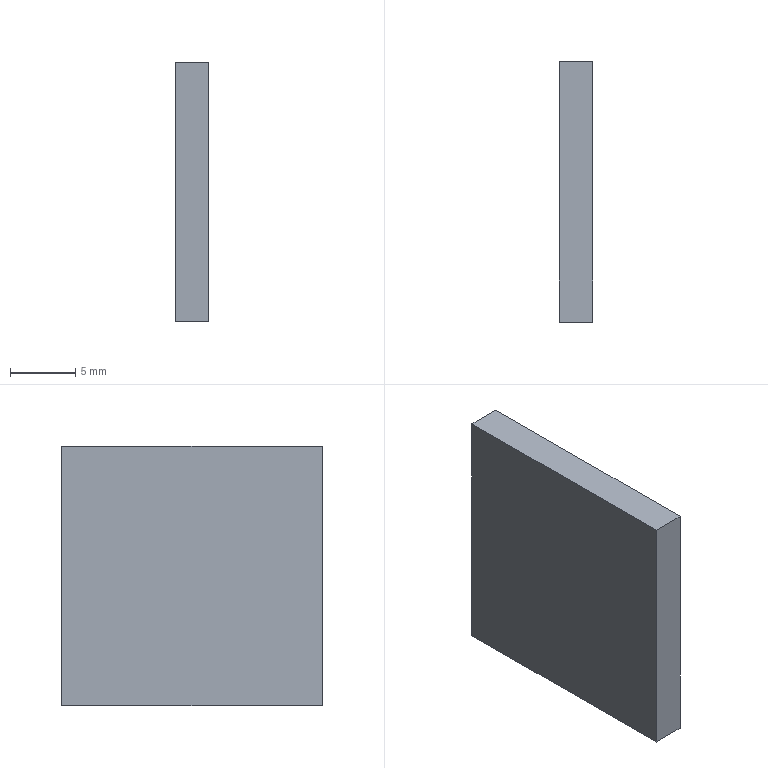Part | NX | features .2 2 | 1 solid | 6 faces | box 2.595 x 20 x 19.901 mm | volume 1033 mm3 | plane 6
STEP:
#1=CARTESIAN_POINT('',(-1240.065,-525.,-424.024));
#2=VERTEX_POINT('',#1);
#3=CARTESIAN_POINT('',(-1240.065,-545.,-424.024));
#4=VERTEX_POINT('',#3);
#5=CARTESIAN_POINT('',(-1240.065,-535.,-424.024));
#6=DIRECTION('',(0.,-1.,0.));
#7=VECTOR('',#6,1000.);
#8=LINE('',#5,#7);
#9=EDGE_CURVE('',#2,#4,#8,.T.);
#10=ORIENTED_EDGE('',*,*,#9,.F.);
#11=CARTESIAN_POINT('',(-1237.47,-525.,-424.024));
#12=VERTEX_POINT('',#11);
#13=CARTESIAN_POINT('',(-1238.768,-525.,-424.024));
#14=DIRECTION('',(1.,0.,0.));
#15=VECTOR('',#14,1000.);
#16=LINE('',#13,#15);
#17=EDGE_CURVE('',#2,#12,#16,.T.);
#18=ORIENTED_EDGE('',*,*,#17,.T.);
#19=CARTESIAN_POINT('',(-1237.47,-545.,-424.024));
#20=VERTEX_POINT('',#19);
#21=CARTESIAN_POINT('',(-1237.47,-535.,-424.024));
#22=DIRECTION('',(0.,-1.,0.));
#23=VECTOR('',#22,1000.);
#24=LINE('',#21,#23);
#25=EDGE_CURVE('',#12,#20,#24,.T.);
#26=ORIENTED_EDGE('',*,*,#25,.T.);
#27=CARTESIAN_POINT('',(-1238.768,-545.,-424.024));
#28=DIRECTION('',(1.,0.,0.));
#29=VECTOR('',#28,1000.);
#30=LINE('',#27,#29);
#31=EDGE_CURVE('',#4,#20,#30,.T.);
#32=ORIENTED_EDGE('',*,*,#31,.F.);
#33=EDGE_LOOP('',(#10,#18,#26,#32));
#34=FACE_BOUND('',#33,.T.);
#35=CARTESIAN_POINT('',(-1237.47,-535.,-424.024));
#36=DIRECTION('',(0.,0.,1.));
#37=DIRECTION('',(-1.,0.,0.));
#38=AXIS2_PLACEMENT_3D('',#35,#36,#37);
#39=PLANE('',#38);
#40=ADVANCED_FACE('',(#34),#39,.F.);
#41=ORIENTED_EDGE('',*,*,#25,.F.);
#42=CARTESIAN_POINT('',(-1237.47,-525.,-404.124));
#43=VERTEX_POINT('',#42);
#44=CARTESIAN_POINT('',(-1237.47,-525.,-414.074));
#45=DIRECTION('',(0.,0.,1.));
#46=VECTOR('',#45,1000.);
#47=LINE('',#44,#46);
#48=EDGE_CURVE('',#12,#43,#47,.T.);
#49=ORIENTED_EDGE('',*,*,#48,.T.);
#50=CARTESIAN_POINT('',(-1237.47,-545.,-404.124));
#51=VERTEX_POINT('',#50);
#52=CARTESIAN_POINT('',(-1237.47,-535.,-404.124));
#53=DIRECTION('',(0.,-1.,0.));
#54=VECTOR('',#53,1000.);
#55=LINE('',#52,#54);
#56=EDGE_CURVE('',#43,#51,#55,.T.);
#57=ORIENTED_EDGE('',*,*,#56,.T.);
#58=CARTESIAN_POINT('',(-1237.47,-545.,-414.074));
#59=DIRECTION('',(0.,0.,1.));
#60=VECTOR('',#59,1000.);
#61=LINE('',#58,#60);
#62=EDGE_CURVE('',#20,#51,#61,.T.);
#63=ORIENTED_EDGE('',*,*,#62,.F.);
#64=EDGE_LOOP('',(#41,#49,#57,#63));
#65=FACE_BOUND('',#64,.T.);
#66=CARTESIAN_POINT('',(-1237.47,-535.,-404.124));
#67=DIRECTION('',(-1.,0.,0.));
#68=DIRECTION('',(0.,0.,-1.));
#69=AXIS2_PLACEMENT_3D('',#66,#67,#68);
#70=PLANE('',#69);
#71=ADVANCED_FACE('',(#65),#70,.F.);
#72=ORIENTED_EDGE('',*,*,#56,.F.);
#73=CARTESIAN_POINT('',(-1240.065,-525.,-404.124));
#74=VERTEX_POINT('',#73);
#75=CARTESIAN_POINT('',(-1238.768,-525.,-404.124));
#76=DIRECTION('',(-1.,0.,0.));
#77=VECTOR('',#76,1000.);
#78=LINE('',#75,#77);
#79=EDGE_CURVE('',#43,#74,#78,.T.);
#80=ORIENTED_EDGE('',*,*,#79,.T.);
#81=CARTESIAN_POINT('',(-1240.065,-545.,-404.124));
#82=VERTEX_POINT('',#81);
#83=CARTESIAN_POINT('',(-1240.065,-535.,-404.124));
#84=DIRECTION('',(0.,-1.,0.));
#85=VECTOR('',#84,1000.);
#86=LINE('',#83,#85);
#87=EDGE_CURVE('',#74,#82,#86,.T.);
#88=ORIENTED_EDGE('',*,*,#87,.T.);
#89=CARTESIAN_POINT('',(-1238.768,-545.,-404.124));
#90=DIRECTION('',(-1.,0.,0.));
#91=VECTOR('',#90,1000.);
#92=LINE('',#89,#91);
#93=EDGE_CURVE('',#51,#82,#92,.T.);
#94=ORIENTED_EDGE('',*,*,#93,.F.);
#95=EDGE_LOOP('',(#72,#80,#88,#94));
#96=FACE_BOUND('',#95,.T.);
#97=CARTESIAN_POINT('',(-1245.159,-535.,-404.124));
#98=DIRECTION('',(0.,0.,-1.));
#99=DIRECTION('',(1.,0.,0.));
#100=AXIS2_PLACEMENT_3D('',#97,#98,#99);
#101=PLANE('',#100);
#102=ADVANCED_FACE('',(#96),#101,.F.);
#103=ORIENTED_EDGE('',*,*,#87,.F.);
#104=CARTESIAN_POINT('',(-1240.065,-525.,-414.074));
#105=DIRECTION('',(0.,0.,-1.));
#106=VECTOR('',#105,1000.);
#107=LINE('',#104,#106);
#108=EDGE_CURVE('',#74,#2,#107,.T.);
#109=ORIENTED_EDGE('',*,*,#108,.T.);
#110=ORIENTED_EDGE('',*,*,#9,.T.);
#111=CARTESIAN_POINT('',(-1240.065,-545.,-414.074));
#112=DIRECTION('',(0.,0.,-1.));
#113=VECTOR('',#112,1000.);
#114=LINE('',#111,#113);
#115=EDGE_CURVE('',#82,#4,#114,.T.);
#116=ORIENTED_EDGE('',*,*,#115,.F.);
#117=EDGE_LOOP('',(#103,#109,#110,#116));
#118=FACE_BOUND('',#117,.T.);
#119=CARTESIAN_POINT('',(-1240.065,-535.,-424.024));
#120=DIRECTION('',(1.,0.,0.));
#121=DIRECTION('',(0.,0.,1.));
#122=AXIS2_PLACEMENT_3D('',#119,#120,#121);
#123=PLANE('',#122);
#124=ADVANCED_FACE('',(#118),#123,.F.);
#125=ORIENTED_EDGE('',*,*,#108,.F.);
#126=ORIENTED_EDGE('',*,*,#79,.F.);
#127=ORIENTED_EDGE('',*,*,#48,.F.);
#128=ORIENTED_EDGE('',*,*,#17,.F.);
#129=EDGE_LOOP('',(#125,#126,#127,#128));
#130=FACE_BOUND('',#129,.T.);
#131=CARTESIAN_POINT('',(-1141.,-525.,-500.));
#132=DIRECTION('',(0.,-1.,0.));
#133=DIRECTION('',(-1.,0.,0.));
#134=AXIS2_PLACEMENT_3D('',#131,#132,#133);
#135=PLANE('',#134);
#136=ADVANCED_FACE('',(#130),#135,.F.);
#137=ORIENTED_EDGE('',*,*,#31,.T.);
#138=ORIENTED_EDGE('',*,*,#62,.T.);
#139=ORIENTED_EDGE('',*,*,#93,.T.);
#140=ORIENTED_EDGE('',*,*,#115,.T.);
#141=EDGE_LOOP('',(#137,#138,#139,#140));
#142=FACE_BOUND('',#141,.T.);
#143=CARTESIAN_POINT('',(-1141.,-545.,-500.));
#144=DIRECTION('',(0.,-1.,0.));
#145=DIRECTION('',(-1.,0.,0.));
#146=AXIS2_PLACEMENT_3D('',#143,#144,#145);
#147=PLANE('',#146);
#148=ADVANCED_FACE('',(#142),#147,.T.);
#149=CLOSED_SHELL('',(#40,#71,#102,#124,#136,#148));
#150=MANIFOLD_SOLID_BREP('',#149);
#151=(LENGTH_UNIT()NAMED_UNIT(*)SI_UNIT(.MILLI.,.METRE.));
#152=UNCERTAINTY_MEASURE_WITH_UNIT(LENGTH_MEASURE(0.00001),#151,'','');
#153=(NAMED_UNIT(*)PLANE_ANGLE_UNIT()SI_UNIT($,.RADIAN.));
#154=(NAMED_UNIT(*)SI_UNIT($,.STERADIAN.)SOLID_ANGLE_UNIT());
#155=(GEOMETRIC_REPRESENTATION_CONTEXT(3)GLOBAL_UNCERTAINTY_ASSIGNED_CONTEXT((#152))GLOBAL_UNIT_ASSIGNED_CONTEXT((#151,#153,#154))REPRESENTATION_CONTEXT('',''));
#156=ADVANCED_BREP_SHAPE_REPRESENTATION('',(#150),#155);